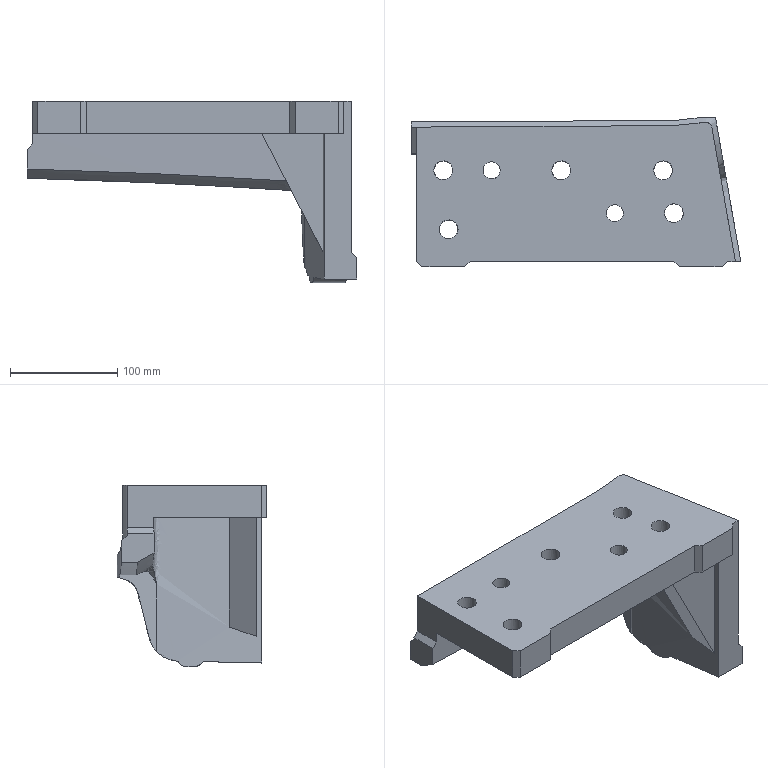Part | NX | features solid 2 | 1 solid | 42 faces | box 307.454 x 140.587 x 169.673 mm | volume 1854465 mm3 | plane 22 | cylinder 12 | spline 8 | commonest cylinder face diameters 17.5 x5 25 x5 16 x2